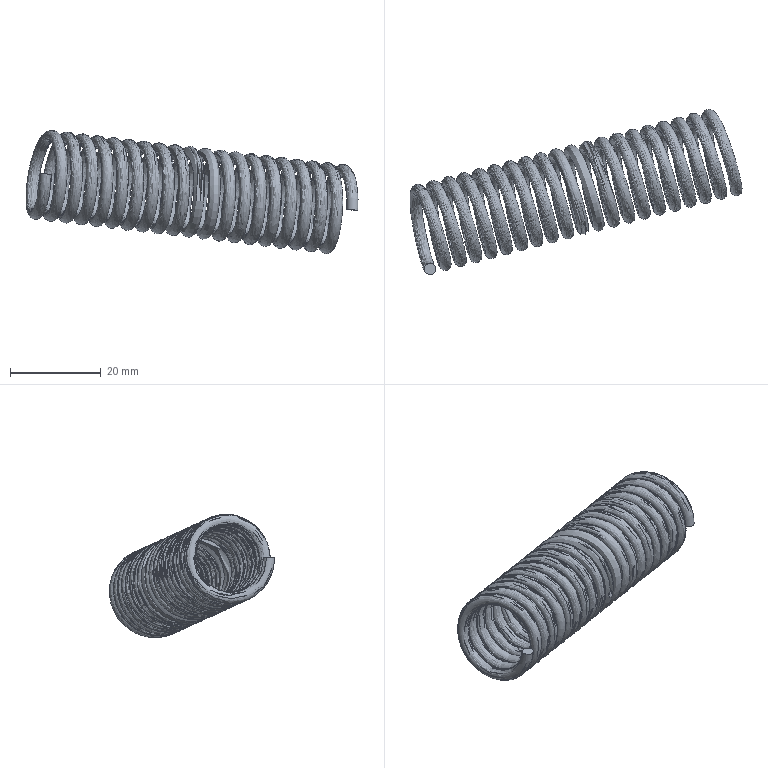Part | STEP file | 车灯-后视镜_id558_x_t | 1 solid | 3 faces | box 73.047 x 36.358 x 27.14 mm | volume 5259 mm3 | plane 2 | spline 1